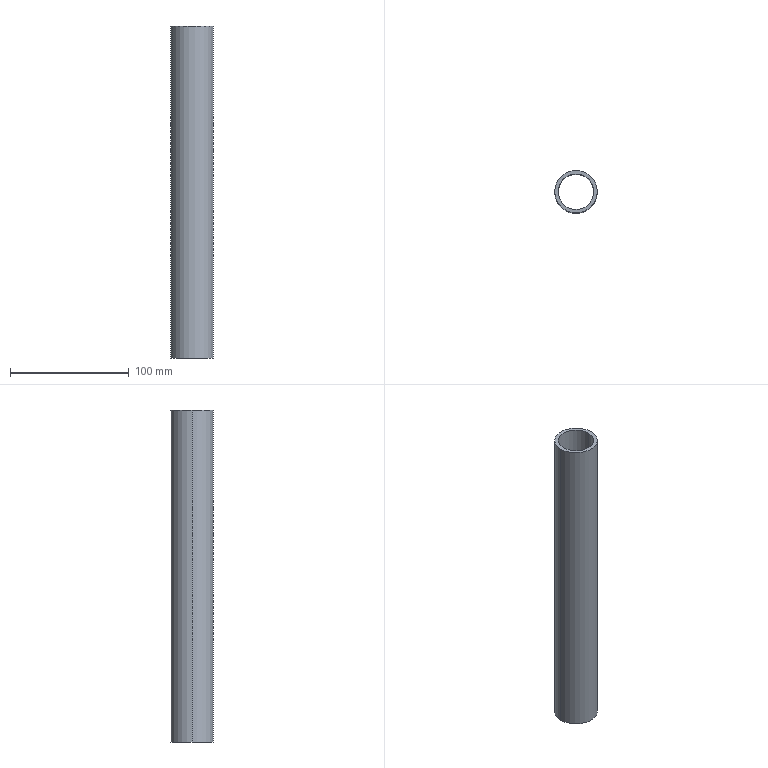Part | STEP file | 1 solid | 6 faces | box 36 x 36 x 280 mm | volume 87085 mm3 | cylinder 4 | plane 2 | commonest cylinder face diameters 30 x2 36 x2
STEP:
#1=CARTESIAN_POINT('',(0.,0.,0.));
#2=DIRECTION('',(0.,0.,1.));
#3=DIRECTION('',(1.,0.,0.));
#4=AXIS2_PLACEMENT_3D('',#1,#2,#3);
#5=CARTESIAN_POINT('',(-15.,0.,140.));
#6=VERTEX_POINT('',#5);
#7=CARTESIAN_POINT('',(-15.,0.,-140.));
#8=VERTEX_POINT('',#7);
#9=CARTESIAN_POINT('',(-15.,0.,140.));
#10=DIRECTION('',(0.,0.,-1.));
#11=VECTOR('',#10,1.);
#12=LINE('',#9,#11);
#13=CARTESIAN_POINT('',(0.,0.,140.));
#14=DIRECTION('',(0.,0.,-1.));
#15=DIRECTION('',(-1.,0.,0.));
#16=AXIS2_PLACEMENT_3D('',#13,#14,#15);
#17=CYLINDRICAL_SURFACE('',#16,15.);
#18=CARTESIAN_POINT('',(6.283,0.));
#19=DIRECTION('',(0.,1.));
#20=VECTOR('',#19,1.);
#21=LINE('',#18,#20);
#22=(GEOMETRIC_REPRESENTATION_CONTEXT(2)PARAMETRIC_REPRESENTATION_CONTEXT()REPRESENTATION_CONTEXT('',''));
#23=DEFINITIONAL_REPRESENTATION('',(#21),#22);
#24=PCURVE('',#17,#23);
#25=CARTESIAN_POINT('',(0.,0.,140.));
#26=DIRECTION('',(0.,0.,-1.));
#27=DIRECTION('',(-1.,0.,0.));
#28=AXIS2_PLACEMENT_3D('',#25,#26,#27);
#29=CYLINDRICAL_SURFACE('',#28,15.);
#30=CARTESIAN_POINT('',(0.,0.));
#31=DIRECTION('',(0.,1.));
#32=VECTOR('',#31,1.);
#33=LINE('',#30,#32);
#34=(GEOMETRIC_REPRESENTATION_CONTEXT(2)PARAMETRIC_REPRESENTATION_CONTEXT()REPRESENTATION_CONTEXT('',''));
#35=DEFINITIONAL_REPRESENTATION('',(#33),#34);
#36=PCURVE('',#29,#35);
#37=SURFACE_CURVE('',#12,(#24,#36),.PCURVE_S1.);
#38=EDGE_CURVE('',#6,#8,#37,.T.);
#39=ORIENTED_EDGE('',*,*,#38,.T.);
#40=CARTESIAN_POINT('',(15.,0.,-140.));
#41=VERTEX_POINT('',#40);
#42=CARTESIAN_POINT('',(0.,0.,-140.));
#43=DIRECTION('',(0.,0.,1.));
#44=DIRECTION('',(1.,0.,0.));
#45=AXIS2_PLACEMENT_3D('',#42,#43,#44);
#46=CIRCLE('',#45,15.);
#47=CARTESIAN_POINT('',(9.425,280.));
#48=DIRECTION('',(-1.,0.));
#49=VECTOR('',#48,1.);
#50=LINE('',#47,#49);
#51=(GEOMETRIC_REPRESENTATION_CONTEXT(2)PARAMETRIC_REPRESENTATION_CONTEXT()REPRESENTATION_CONTEXT('',''));
#52=DEFINITIONAL_REPRESENTATION('',(#50),#51);
#53=PCURVE('',#17,#52);
#54=CARTESIAN_POINT('',(0.,0.,-140.));
#55=DIRECTION('',(0.,0.,1.));
#56=DIRECTION('',(1.,0.,0.));
#57=AXIS2_PLACEMENT_3D('',#54,#55,#56);
#58=PLANE('',#57);
#59=CARTESIAN_POINT('',(0.,0.));
#60=DIRECTION('',(1.,0.));
#61=AXIS2_PLACEMENT_2D('',#59,#60);
#62=CIRCLE('',#61,15.);
#63=(GEOMETRIC_REPRESENTATION_CONTEXT(2)PARAMETRIC_REPRESENTATION_CONTEXT()REPRESENTATION_CONTEXT('',''));
#64=DEFINITIONAL_REPRESENTATION('',(#62),#63);
#65=PCURVE('',#58,#64);
#66=SURFACE_CURVE('',#46,(#53,#65),.PCURVE_S1.);
#67=EDGE_CURVE('',#8,#41,#66,.T.);
#68=ORIENTED_EDGE('',*,*,#67,.T.);
#69=CARTESIAN_POINT('',(15.,0.,140.));
#70=VERTEX_POINT('',#69);
#71=CARTESIAN_POINT('',(15.,0.,140.));
#72=DIRECTION('',(0.,0.,-1.));
#73=VECTOR('',#72,1.);
#74=LINE('',#71,#73);
#75=CARTESIAN_POINT('',(3.142,0.));
#76=DIRECTION('',(0.,1.));
#77=VECTOR('',#76,1.);
#78=LINE('',#75,#77);
#79=(GEOMETRIC_REPRESENTATION_CONTEXT(2)PARAMETRIC_REPRESENTATION_CONTEXT()REPRESENTATION_CONTEXT('',''));
#80=DEFINITIONAL_REPRESENTATION('',(#78),#79);
#81=PCURVE('',#17,#80);
#82=CARTESIAN_POINT('',(3.142,0.));
#83=DIRECTION('',(0.,1.));
#84=VECTOR('',#83,1.);
#85=LINE('',#82,#84);
#86=(GEOMETRIC_REPRESENTATION_CONTEXT(2)PARAMETRIC_REPRESENTATION_CONTEXT()REPRESENTATION_CONTEXT('',''));
#87=DEFINITIONAL_REPRESENTATION('',(#85),#86);
#88=PCURVE('',#29,#87);
#89=SURFACE_CURVE('',#74,(#81,#88),.PCURVE_S1.);
#90=EDGE_CURVE('',#70,#41,#89,.T.);
#91=ORIENTED_EDGE('',*,*,#90,.F.);
#92=CARTESIAN_POINT('',(0.,0.,140.));
#93=DIRECTION('',(0.,0.,1.));
#94=DIRECTION('',(1.,0.,0.));
#95=AXIS2_PLACEMENT_3D('',#92,#93,#94);
#96=CIRCLE('',#95,15.);
#97=CARTESIAN_POINT('',(9.425,0.));
#98=DIRECTION('',(-1.,0.));
#99=VECTOR('',#98,1.);
#100=LINE('',#97,#99);
#101=(GEOMETRIC_REPRESENTATION_CONTEXT(2)PARAMETRIC_REPRESENTATION_CONTEXT()REPRESENTATION_CONTEXT('',''));
#102=DEFINITIONAL_REPRESENTATION('',(#100),#101);
#103=PCURVE('',#17,#102);
#104=CARTESIAN_POINT('',(0.,0.,140.));
#105=DIRECTION('',(0.,0.,1.));
#106=DIRECTION('',(1.,0.,0.));
#107=AXIS2_PLACEMENT_3D('',#104,#105,#106);
#108=PLANE('',#107);
#109=CARTESIAN_POINT('',(0.,0.));
#110=DIRECTION('',(1.,0.));
#111=AXIS2_PLACEMENT_2D('',#109,#110);
#112=CIRCLE('',#111,15.);
#113=(GEOMETRIC_REPRESENTATION_CONTEXT(2)PARAMETRIC_REPRESENTATION_CONTEXT()REPRESENTATION_CONTEXT('',''));
#114=DEFINITIONAL_REPRESENTATION('',(#112),#113);
#115=PCURVE('',#108,#114);
#116=SURFACE_CURVE('',#96,(#103,#115),.PCURVE_S1.);
#117=EDGE_CURVE('',#6,#70,#116,.T.);
#118=ORIENTED_EDGE('',*,*,#117,.F.);
#119=EDGE_LOOP('',(#39,#68,#91,#118));
#120=FACE_BOUND('',#119,.F.);
#121=ADVANCED_FACE('',(#120),#17,.F.);
#122=CARTESIAN_POINT('',(18.,0.,140.));
#123=VERTEX_POINT('',#122);
#124=CARTESIAN_POINT('',(-18.,0.,140.));
#125=VERTEX_POINT('',#124);
#126=CARTESIAN_POINT('',(0.,0.,140.));
#127=DIRECTION('',(0.,0.,1.));
#128=DIRECTION('',(1.,0.,0.));
#129=AXIS2_PLACEMENT_3D('',#126,#127,#128);
#130=CIRCLE('',#129,18.);
#131=CARTESIAN_POINT('',(0.,0.,140.));
#132=DIRECTION('',(0.,0.,-1.));
#133=DIRECTION('',(-1.,0.,0.));
#134=AXIS2_PLACEMENT_3D('',#131,#132,#133);
#135=CYLINDRICAL_SURFACE('',#134,18.);
#136=CARTESIAN_POINT('',(3.142,0.));
#137=DIRECTION('',(-1.,0.));
#138=VECTOR('',#137,1.);
#139=LINE('',#136,#138);
#140=(GEOMETRIC_REPRESENTATION_CONTEXT(2)PARAMETRIC_REPRESENTATION_CONTEXT()REPRESENTATION_CONTEXT('',''));
#141=DEFINITIONAL_REPRESENTATION('',(#139),#140);
#142=PCURVE('',#135,#141);
#143=CARTESIAN_POINT('',(0.,0.));
#144=DIRECTION('',(1.,0.));
#145=AXIS2_PLACEMENT_2D('',#143,#144);
#146=CIRCLE('',#145,18.);
#147=(GEOMETRIC_REPRESENTATION_CONTEXT(2)PARAMETRIC_REPRESENTATION_CONTEXT()REPRESENTATION_CONTEXT('',''));
#148=DEFINITIONAL_REPRESENTATION('',(#146),#147);
#149=PCURVE('',#108,#148);
#150=SURFACE_CURVE('',#130,(#142,#149),.PCURVE_S1.);
#151=EDGE_CURVE('',#123,#125,#150,.T.);
#152=ORIENTED_EDGE('',*,*,#151,.F.);
#153=CARTESIAN_POINT('',(18.,0.,-140.));
#154=VERTEX_POINT('',#153);
#155=CARTESIAN_POINT('',(18.,0.,140.));
#156=DIRECTION('',(0.,0.,-1.));
#157=VECTOR('',#156,1.);
#158=LINE('',#155,#157);
#159=CARTESIAN_POINT('',(3.142,0.));
#160=DIRECTION('',(0.,1.));
#161=VECTOR('',#160,1.);
#162=LINE('',#159,#161);
#163=(GEOMETRIC_REPRESENTATION_CONTEXT(2)PARAMETRIC_REPRESENTATION_CONTEXT()REPRESENTATION_CONTEXT('',''));
#164=DEFINITIONAL_REPRESENTATION('',(#162),#163);
#165=PCURVE('',#135,#164);
#166=CARTESIAN_POINT('',(0.,0.,140.));
#167=DIRECTION('',(0.,0.,-1.));
#168=DIRECTION('',(-1.,0.,0.));
#169=AXIS2_PLACEMENT_3D('',#166,#167,#168);
#170=CYLINDRICAL_SURFACE('',#169,18.);
#171=CARTESIAN_POINT('',(3.142,0.));
#172=DIRECTION('',(0.,1.));
#173=VECTOR('',#172,1.);
#174=LINE('',#171,#173);
#175=(GEOMETRIC_REPRESENTATION_CONTEXT(2)PARAMETRIC_REPRESENTATION_CONTEXT()REPRESENTATION_CONTEXT('',''));
#176=DEFINITIONAL_REPRESENTATION('',(#174),#175);
#177=PCURVE('',#170,#176);
#178=SURFACE_CURVE('',#158,(#165,#177),.PCURVE_S1.);
#179=EDGE_CURVE('',#123,#154,#178,.T.);
#180=ORIENTED_EDGE('',*,*,#179,.T.);
#181=CARTESIAN_POINT('',(-18.,0.,-140.));
#182=VERTEX_POINT('',#181);
#183=CARTESIAN_POINT('',(0.,0.,-140.));
#184=DIRECTION('',(0.,0.,1.));
#185=DIRECTION('',(1.,0.,0.));
#186=AXIS2_PLACEMENT_3D('',#183,#184,#185);
#187=CIRCLE('',#186,18.);
#188=CARTESIAN_POINT('',(3.142,280.));
#189=DIRECTION('',(-1.,0.));
#190=VECTOR('',#189,1.);
#191=LINE('',#188,#190);
#192=(GEOMETRIC_REPRESENTATION_CONTEXT(2)PARAMETRIC_REPRESENTATION_CONTEXT()REPRESENTATION_CONTEXT('',''));
#193=DEFINITIONAL_REPRESENTATION('',(#191),#192);
#194=PCURVE('',#135,#193);
#195=CARTESIAN_POINT('',(0.,0.));
#196=DIRECTION('',(1.,0.));
#197=AXIS2_PLACEMENT_2D('',#195,#196);
#198=CIRCLE('',#197,18.);
#199=(GEOMETRIC_REPRESENTATION_CONTEXT(2)PARAMETRIC_REPRESENTATION_CONTEXT()REPRESENTATION_CONTEXT('',''));
#200=DEFINITIONAL_REPRESENTATION('',(#198),#199);
#201=PCURVE('',#58,#200);
#202=SURFACE_CURVE('',#187,(#194,#201),.PCURVE_S1.);
#203=EDGE_CURVE('',#154,#182,#202,.T.);
#204=ORIENTED_EDGE('',*,*,#203,.T.);
#205=CARTESIAN_POINT('',(-18.,0.,140.));
#206=DIRECTION('',(0.,0.,-1.));
#207=VECTOR('',#206,1.);
#208=LINE('',#205,#207);
#209=CARTESIAN_POINT('',(0.,0.));
#210=DIRECTION('',(0.,1.));
#211=VECTOR('',#210,1.);
#212=LINE('',#209,#211);
#213=(GEOMETRIC_REPRESENTATION_CONTEXT(2)PARAMETRIC_REPRESENTATION_CONTEXT()REPRESENTATION_CONTEXT('',''));
#214=DEFINITIONAL_REPRESENTATION('',(#212),#213);
#215=PCURVE('',#135,#214);
#216=CARTESIAN_POINT('',(6.283,0.));
#217=DIRECTION('',(0.,1.));
#218=VECTOR('',#217,1.);
#219=LINE('',#216,#218);
#220=(GEOMETRIC_REPRESENTATION_CONTEXT(2)PARAMETRIC_REPRESENTATION_CONTEXT()REPRESENTATION_CONTEXT('',''));
#221=DEFINITIONAL_REPRESENTATION('',(#219),#220);
#222=PCURVE('',#170,#221);
#223=SURFACE_CURVE('',#208,(#215,#222),.PCURVE_S1.);
#224=EDGE_CURVE('',#125,#182,#223,.T.);
#225=ORIENTED_EDGE('',*,*,#224,.F.);
#226=EDGE_LOOP('',(#152,#180,#204,#225));
#227=FACE_BOUND('',#226,.T.);
#228=ADVANCED_FACE('',(#227),#135,.T.);
#229=CARTESIAN_POINT('',(0.,0.,140.));
#230=DIRECTION('',(0.,0.,1.));
#231=DIRECTION('',(1.,0.,0.));
#232=AXIS2_PLACEMENT_3D('',#229,#230,#231);
#233=CIRCLE('',#232,18.);
#234=CARTESIAN_POINT('',(0.,0.));
#235=DIRECTION('',(1.,0.));
#236=AXIS2_PLACEMENT_2D('',#234,#235);
#237=CIRCLE('',#236,18.);
#238=(GEOMETRIC_REPRESENTATION_CONTEXT(2)PARAMETRIC_REPRESENTATION_CONTEXT()REPRESENTATION_CONTEXT('',''));
#239=DEFINITIONAL_REPRESENTATION('',(#237),#238);
#240=PCURVE('',#108,#239);
#241=CARTESIAN_POINT('',(9.425,0.));
#242=DIRECTION('',(-1.,0.));
#243=VECTOR('',#242,1.);
#244=LINE('',#241,#243);
#245=(GEOMETRIC_REPRESENTATION_CONTEXT(2)PARAMETRIC_REPRESENTATION_CONTEXT()REPRESENTATION_CONTEXT('',''));
#246=DEFINITIONAL_REPRESENTATION('',(#244),#245);
#247=PCURVE('',#170,#246);
#248=SURFACE_CURVE('',#233,(#240,#247),.PCURVE_S1.);
#249=EDGE_CURVE('',#125,#123,#248,.T.);
#250=ORIENTED_EDGE('',*,*,#249,.T.);
#251=ORIENTED_EDGE('',*,*,#151,.T.);
#252=EDGE_LOOP('',(#250,#251));
#253=FACE_BOUND('',#252,.T.);
#254=ORIENTED_EDGE('',*,*,#117,.F.);
#255=CARTESIAN_POINT('',(0.,0.,140.));
#256=DIRECTION('',(0.,0.,1.));
#257=DIRECTION('',(1.,0.,0.));
#258=AXIS2_PLACEMENT_3D('',#255,#256,#257);
#259=CIRCLE('',#258,15.);
#260=CARTESIAN_POINT('',(0.,0.));
#261=DIRECTION('',(1.,0.));
#262=AXIS2_PLACEMENT_2D('',#260,#261);
#263=CIRCLE('',#262,15.);
#264=(GEOMETRIC_REPRESENTATION_CONTEXT(2)PARAMETRIC_REPRESENTATION_CONTEXT()REPRESENTATION_CONTEXT('',''));
#265=DEFINITIONAL_REPRESENTATION('',(#263),#264);
#266=PCURVE('',#108,#265);
#267=CARTESIAN_POINT('',(3.142,0.));
#268=DIRECTION('',(-1.,0.));
#269=VECTOR('',#268,1.);
#270=LINE('',#267,#269);
#271=(GEOMETRIC_REPRESENTATION_CONTEXT(2)PARAMETRIC_REPRESENTATION_CONTEXT()REPRESENTATION_CONTEXT('',''));
#272=DEFINITIONAL_REPRESENTATION('',(#270),#271);
#273=PCURVE('',#29,#272);
#274=SURFACE_CURVE('',#259,(#266,#273),.PCURVE_S1.);
#275=EDGE_CURVE('',#70,#6,#274,.T.);
#276=ORIENTED_EDGE('',*,*,#275,.F.);
#277=EDGE_LOOP('',(#254,#276));
#278=FACE_BOUND('',#277,.T.);
#279=ADVANCED_FACE('',(#253,#278),#108,.T.);
#280=CARTESIAN_POINT('',(0.,0.,-140.));
#281=DIRECTION('',(0.,0.,1.));
#282=DIRECTION('',(1.,0.,0.));
#283=AXIS2_PLACEMENT_3D('',#280,#281,#282);
#284=CIRCLE('',#283,18.);
#285=CARTESIAN_POINT('',(0.,0.));
#286=DIRECTION('',(1.,0.));
#287=AXIS2_PLACEMENT_2D('',#285,#286);
#288=CIRCLE('',#287,18.);
#289=(GEOMETRIC_REPRESENTATION_CONTEXT(2)PARAMETRIC_REPRESENTATION_CONTEXT()REPRESENTATION_CONTEXT('',''));
#290=DEFINITIONAL_REPRESENTATION('',(#288),#289);
#291=PCURVE('',#58,#290);
#292=CARTESIAN_POINT('',(9.425,280.));
#293=DIRECTION('',(-1.,0.));
#294=VECTOR('',#293,1.);
#295=LINE('',#292,#294);
#296=(GEOMETRIC_REPRESENTATION_CONTEXT(2)PARAMETRIC_REPRESENTATION_CONTEXT()REPRESENTATION_CONTEXT('',''));
#297=DEFINITIONAL_REPRESENTATION('',(#295),#296);
#298=PCURVE('',#170,#297);
#299=SURFACE_CURVE('',#284,(#291,#298),.PCURVE_S1.);
#300=EDGE_CURVE('',#182,#154,#299,.T.);
#301=ORIENTED_EDGE('',*,*,#300,.F.);
#302=ORIENTED_EDGE('',*,*,#203,.F.);
#303=EDGE_LOOP('',(#301,#302));
#304=FACE_BOUND('',#303,.T.);
#305=ORIENTED_EDGE('',*,*,#67,.T.);
#306=CARTESIAN_POINT('',(0.,0.,-140.));
#307=DIRECTION('',(0.,0.,1.));
#308=DIRECTION('',(1.,0.,0.));
#309=AXIS2_PLACEMENT_3D('',#306,#307,#308);
#310=CIRCLE('',#309,15.);
#311=CARTESIAN_POINT('',(0.,0.));
#312=DIRECTION('',(1.,0.));
#313=AXIS2_PLACEMENT_2D('',#311,#312);
#314=CIRCLE('',#313,15.);
#315=(GEOMETRIC_REPRESENTATION_CONTEXT(2)PARAMETRIC_REPRESENTATION_CONTEXT()REPRESENTATION_CONTEXT('',''));
#316=DEFINITIONAL_REPRESENTATION('',(#314),#315);
#317=PCURVE('',#58,#316);
#318=CARTESIAN_POINT('',(3.142,280.));
#319=DIRECTION('',(-1.,0.));
#320=VECTOR('',#319,1.);
#321=LINE('',#318,#320);
#322=(GEOMETRIC_REPRESENTATION_CONTEXT(2)PARAMETRIC_REPRESENTATION_CONTEXT()REPRESENTATION_CONTEXT('',''));
#323=DEFINITIONAL_REPRESENTATION('',(#321),#322);
#324=PCURVE('',#29,#323);
#325=SURFACE_CURVE('',#310,(#317,#324),.PCURVE_S1.);
#326=EDGE_CURVE('',#41,#8,#325,.T.);
#327=ORIENTED_EDGE('',*,*,#326,.T.);
#328=EDGE_LOOP('',(#305,#327));
#329=FACE_BOUND('',#328,.T.);
#330=ADVANCED_FACE('',(#304,#329),#58,.F.);
#331=ORIENTED_EDGE('',*,*,#179,.F.);
#332=ORIENTED_EDGE('',*,*,#249,.F.);
#333=ORIENTED_EDGE('',*,*,#224,.T.);
#334=ORIENTED_EDGE('',*,*,#300,.T.);
#335=EDGE_LOOP('',(#331,#332,#333,#334));
#336=FACE_BOUND('',#335,.T.);
#337=ADVANCED_FACE('',(#336),#170,.T.);
#338=ORIENTED_EDGE('',*,*,#326,.T.);
#339=ORIENTED_EDGE('',*,*,#38,.F.);
#340=ORIENTED_EDGE('',*,*,#275,.F.);
#341=ORIENTED_EDGE('',*,*,#90,.T.);
#342=EDGE_LOOP('',(#338,#339,#340,#341));
#343=FACE_BOUND('',#342,.F.);
#344=ADVANCED_FACE('',(#343),#29,.F.);
#345=CLOSED_SHELL('',(#121,#228,#279,#330,#337,#344));
#346=MANIFOLD_SOLID_BREP('',#345);
#347=(LENGTH_UNIT()NAMED_UNIT(*)SI_UNIT(.MILLI.,.METRE.));
#348=UNCERTAINTY_MEASURE_WITH_UNIT(LENGTH_MEASURE(0.0000001),#347,'','');
#349=(NAMED_UNIT(*)PLANE_ANGLE_UNIT()SI_UNIT($,.RADIAN.));
#350=(NAMED_UNIT(*)SI_UNIT($,.STERADIAN.)SOLID_ANGLE_UNIT());
#351=(GEOMETRIC_REPRESENTATION_CONTEXT(3)GLOBAL_UNCERTAINTY_ASSIGNED_CONTEXT((#348))GLOBAL_UNIT_ASSIGNED_CONTEXT((#347,#349,#350))REPRESENTATION_CONTEXT('',''));
#352=ADVANCED_BREP_SHAPE_REPRESENTATION('',(#4,#346),#351);